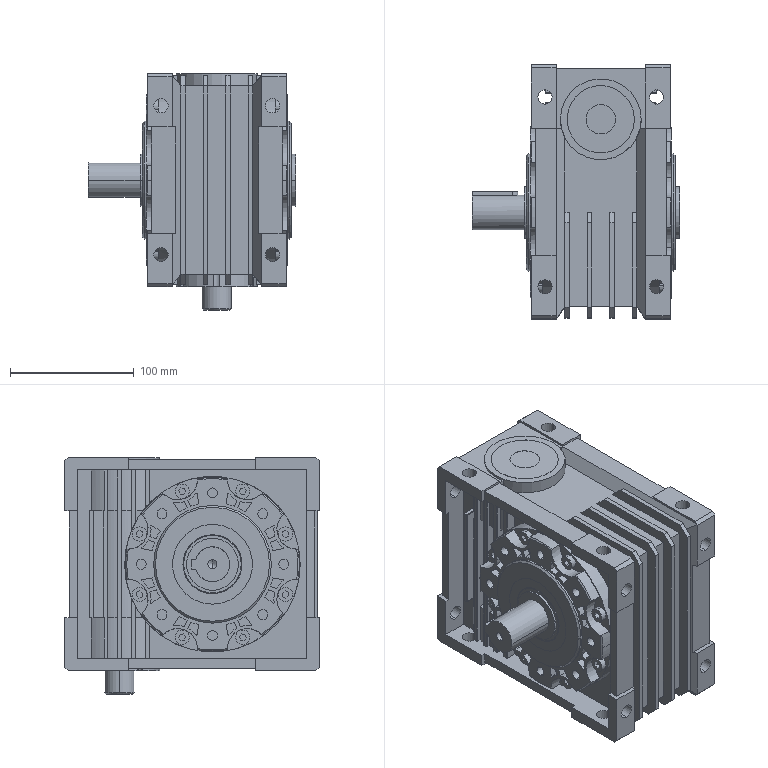Part | SolidWorks | 4 solids | 924 faces | box 167 x 205 x 191 mm | volume 3156838 mm3 | plane 488 | cylinder 380 | cone 56 | commonest cylinder face diameters 1 x80 11.5 x64 36.765 x36 8 x34 99.75 x32 32.015 x24